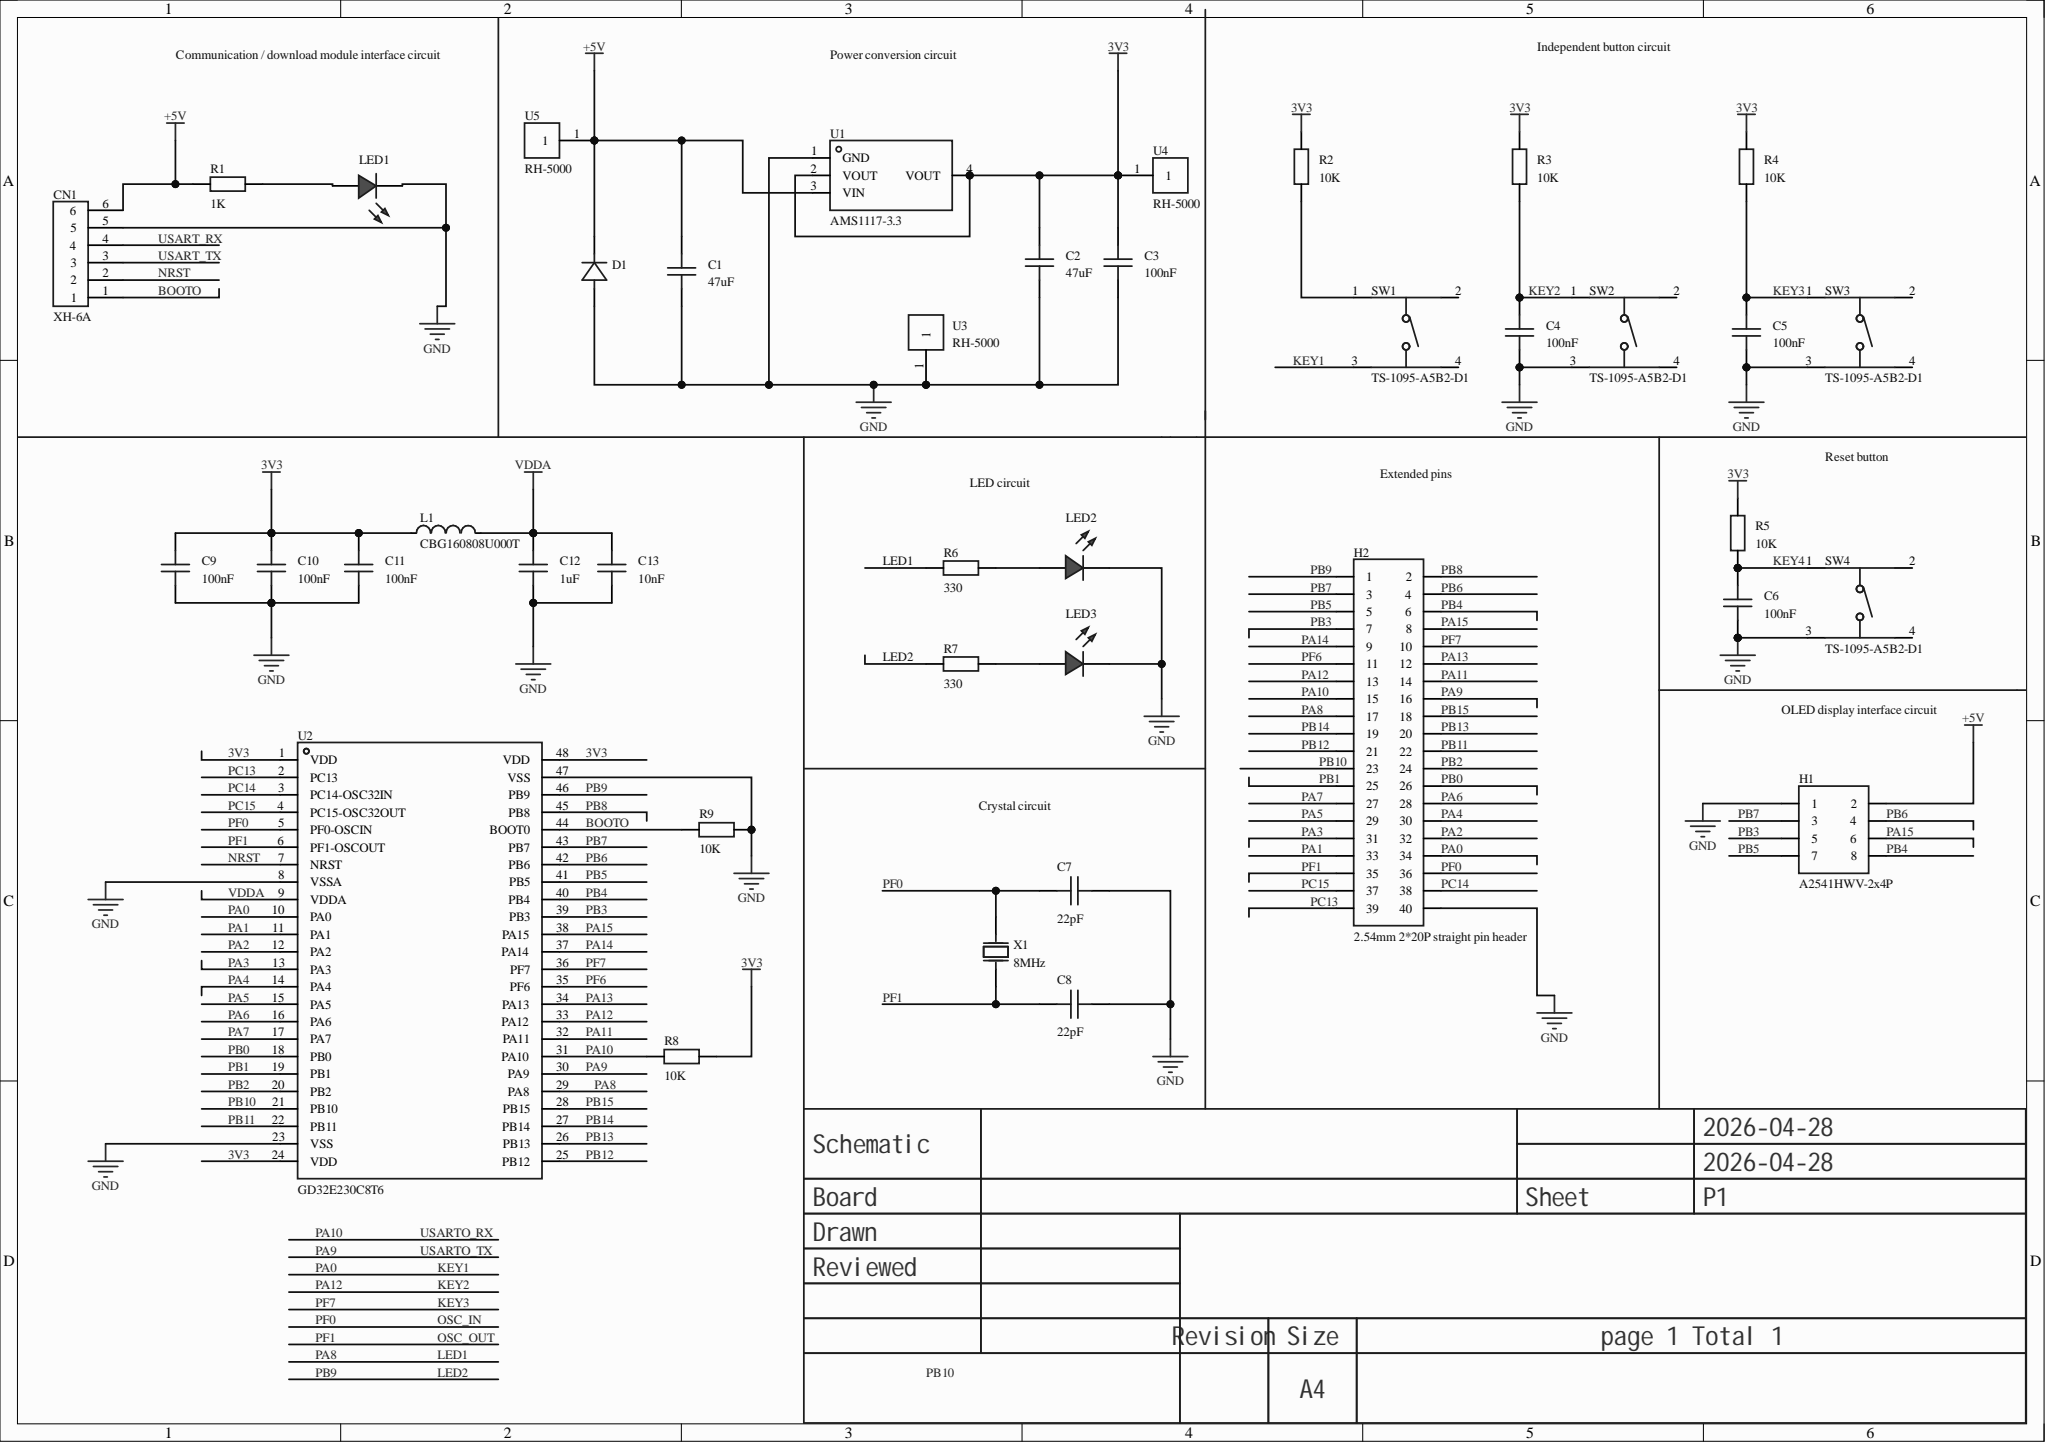Circuit board | Altium Designer | 40 parts | 50 nets
Bill of materials:
Comment,Description,Designator,Footprint,LibRef,Quantity
"47uF","","C1, C2","C0603","CAP_0603","2"
"100nF","","C3, C4, C5, C6, C9, C10, C11","C0603","CAP_0603","7"
"22pF","","C7, C8","C0603","CAP_0603","2"
"1uF","","C12","C0603","CAP_0603","1"
"10nF","","C13","C0603","CAP_0603","1"
"XH-6A","Pin structure: 1x6P; pitch: 2.5mm; mounting: through-hole; reference series: XH; total PIN count: 6P; rows: 1; pins per row: 6; row pitch: -; rated current: -; contact material: -; contact plating: -; operating temperature: -;","CN1","CONN-TH_6P-P2.50_XH-6A","XH-6A_C5663","1"
"","","D1","DO_1N4007","D_1N4007A","1"
"A2541HWV-2x4P","Socket structure: 2x4P; pitch: 2.54mm; row pitch: 2.54mm; round/square hole: square hole; mounting: through-hole; rows: double row; total hole count: 8P; rated current: 3A; rated voltage: 250V; socket direction: top; plastic height: 8.5mm; contact material: brass; contact plating: gold; operating temperature: -40℃~+105℃;","H1","HDR-TH_8P-P2.54-V-F-R2-C4-S2.54-1","A2541HWV-2x4P","1"
"2.54mm 2*20P straight pin header","Pin structure: 2x20P; pitch: 2.54mm; row pitch: 2.54mm; round/square pin: square pin; mounting: through-hole; rows: double row; total PIN count: 40P; rated current: 3A; rated voltage: -; mating pin length: 6mm; plastic height: -; tail length: 3mm; contact material: brass; contact plating: -; operating temperature: -40℃~+105℃; color: black;","H2","HDR-TH_40P-P2.54-V-M-R2-C20-S2.54","2.54mm 2*20P直排针","1"
"CBG160808U000T","Impedance@frequency: 0O@100MHz; DC resistance (DCR): 100mO;","L1","L0603","CBG160808U000T","1"
"","","LED1, LED2, LED3","LED_TH-3mm","LED_TH-R_3mm","3"
"1K","","R1","R0603","Res_0603","1"
"10K","","R2, R3, R4, R5, R8, R9","R0603","Res_0603","6"
"330","","R6, R7","R0603","Res_0603","2"
"TS-1095-A5B2-D1","Circuit structure: SPST; button shape: round button; actuating force: 180gf; mounting: through-hole; switch length: 6mm; switch width: 6mm; switch height: 6mm; bracket: none; mechanical life: -;","SW1, SW2, SW3, SW4","SW-TH_4P-L6.0-W6.0-P4.50-LS6.5","TS-1095-A5B2-D1","4"
"AMS1117-3.3","Output type: fixed; working voltage: 15V; output voltage: 3.3V; output current: 1A; ripple rejection (PSRR): 72dB@(120Hz); output polarity: positive;","U1","SOT-223-3_L6.5-W3.4-P2.30-LS7.0-BR","AMS1117-3.3_C6186","1"
"GD32E230C8T6","CPU core: ARM-M series; max CPU frequency: 72MHz; application field: -;","U2","LQFP-48_L7.0-W7.0-P0.50-LS9.0-BL","GD32E230C8T6","1"
"RH-5000","","U3, U4, U5","TEST-TH_BD2.54-P1.4_RED","RH-5000","3"
"8MHz","Crystal type: SMD crystal; frequency: 8MHz; frequency tolerance at room temperature: ±20ppm; load capacitance: 20pF; frequency stability: ±30ppm;","X1","CRYSTAL-SMD_L11.5-W4.8-LS12.7","X49SM8MSD2SC","1"
Netlist (Protel format):
[
C1
C0603
47uF



]
[
C2
C0603
47uF



]
[
C3
C0603
100nF



]
[
C4
C0603
100nF



]
[
C5
C0603
100nF



]
[
C6
C0603
100nF



]
[
C7
C0603
22pF



]
[
C8
C0603
22pF



]
[
C9
C0603
100nF



]
[
C10
C0603
100nF



]
[
C11
C0603
100nF



]
[
C12
C0603
1uF



]
[
C13
C0603
10nF



]
[
CN1
CONN-TH_6P-P2.50_XH-6A
XH-6A



]
[
D1
DO_1N4007




]
[
H1
HDR-TH_8P-P2.54-V-F-R2-C4-S2.54-1
A2541HWV-2x4P



]
[
H2
HDR-TH_40P-P2.54-V-M-R2-C20-S2.54
2.54mm 2*20P straight pin header



]
[
L1
L0603
CBG160808U000T



]
[
LED1
LED_TH-3mm




]
[
LED2
LED_TH-3mm




]
[
LED3
LED_TH-3mm




]
[
R1
R0603
1K



]
[
R2
R0603
10K



]
[
R3
R0603
10K



]
[
R4
R0603
10K



]
[
R5
R0603
10K



]
[
R6
R0603
330



]
[
R7
R0603
330



]
[
R8
R0603
10K



]
[
R9
R0603
10K



]
[
SW1
SW-TH_4P-L6.0-W6.0-P4.50-LS6.5
TS-1095-A5B2-D1



]
[
SW2
SW-TH_4P-L6.0-W6.0-P4.50-LS6.5
TS-1095-A5B2-D1



]
[
SW3
SW-TH_4P-L6.0-W6.0-P4.50-LS6.5
TS-1095-A5B2-D1



]
[
SW4
SW-TH_4P-L6.0-W6.0-P4.50-LS6.5
TS-1095-A5B2-D1



]
[
U1
SOT-223-3_L6.5-W3.4-P2.30-LS7.0-BR
AMS1117-3.3



]
[
U2
LQFP-48_L7.0-W7.0-P0.50-LS9.0-BL
GD32E230C8T6



]
[
U3
TEST-TH_BD2.54-P1.4_RED
RH-5000



]
[
U4
TEST-TH_BD2.54-P1.4_RED
RH-5000



]
[
U5
TEST-TH_BD2.54-P1.4_RED
RH-5000



]
[
X1
CRYSTAL-SMD_L11.5-W4.8-LS12.7
8MHz



]
(
VDDA
C12-2
C13-2
L1-2
U2-9
)
(
PF6
H2-11
U2-35
)
(
PC15
H2-37
U2-4
)
(
PC14
H2-38
U2-3
)
(
PC13
H2-39
U2-2
)
(
PB15
H2-18
U2-28
)
(
PB14
H2-19
U2-27
)
(
PB13
H2-20
U2-26
)
(
PB12
H2-21
U2-25
)
(
PB11
H2-22
U2-22
)
(
PB10
H2-23
U2-21
)
(
PB8
H2-2
U2-45
)
(
PB7
H1-3
H2-3
U2-43
)
(
PB6
H1-4
H2-4
U2-42
)
(
PB5
H1-7
H2-5
U2-41
)
(
PB4
H1-8
H2-6
U2-40
)
(
PB3
H1-5
H2-7
U2-39
)
(
PB2
H2-24
U2-20
)
(
PB1
H2-25
U2-19
)
(
PB0
H2-26
U2-18
)
(
PA15
H1-6
H2-8
U2-38
)
(
PA14
H2-9
U2-37
)
(
PA13
H2-12
U2-34
)
(
PA11
H2-14
U2-32
)
(
PA10
H2-15
R8-1
U2-31
)
(
PA9
H2-16
U2-30
)
(
PA7
H2-27
U2-17
)
(
PA6
H2-28
U2-16
)
(
PA5
H2-29
U2-15
)
(
PA4
H2-30
U2-14
)
(
PA3
H2-31
U2-13
)
(
PA2
H2-32
U2-12
)
(
PA1
H2-33
U2-11
)
(
OSC_OUT
C8-1
H2-35
U2-6
X1-2
)
(
OSC_IN
C7-1
H2-36
U2-5
X1-1
)
(
NRST
CN1-2
U2-7
)
(
NetR2_1
R2-1
SW1-1
)
(
NetLED3_1
LED3-1
R7-2
)
(
NetLED2_1
LED2-1
R6-2
)
(
NetLED1_1
LED1-1
R1-2
)
(
LED2
H2-1
U2-46
)
(
LED1
H2-17
U2-29
)
(
KEY4
C6-2
R5-1
SW4-1
)
(
KEY3
C5-2
H2-10
R4-1
SW3-1
U2-36
)
(
KEY2
C4-2
H2-13
R3-1
SW2-1
U2-33
)
(
KEY1
H2-34
SW1-3
U2-10
)
(
GND
C1-1
C2-1
C3-1
C4-1
C5-1
C6-1
C7-2
C8-2
C9-1
C10-1
C11-1
C12-1
C13-1
CN1-5
D1-2
H1-1
H2-40
LED1-2
LED2-2
LED3-2
R9-2
SW2-3
SW3-3
SW4-3
U1-1
U2-8
U2-23
U2-47
U3-1
)
(
BOOTO
CN1-1
R9-1
U2-44
)
(
+5V
C1-2
CN1-6
D1-1
H1-2
R1-1
U1-3
U5-1
)
(
3V3
C2-2
C3-2
C9-2
C10-2
C11-2
L1-1
R2-2
R3-2
R4-2
R5-2
R8-2
U1-2
U1-4
U2-1
U2-24
U2-48
U4-1
)